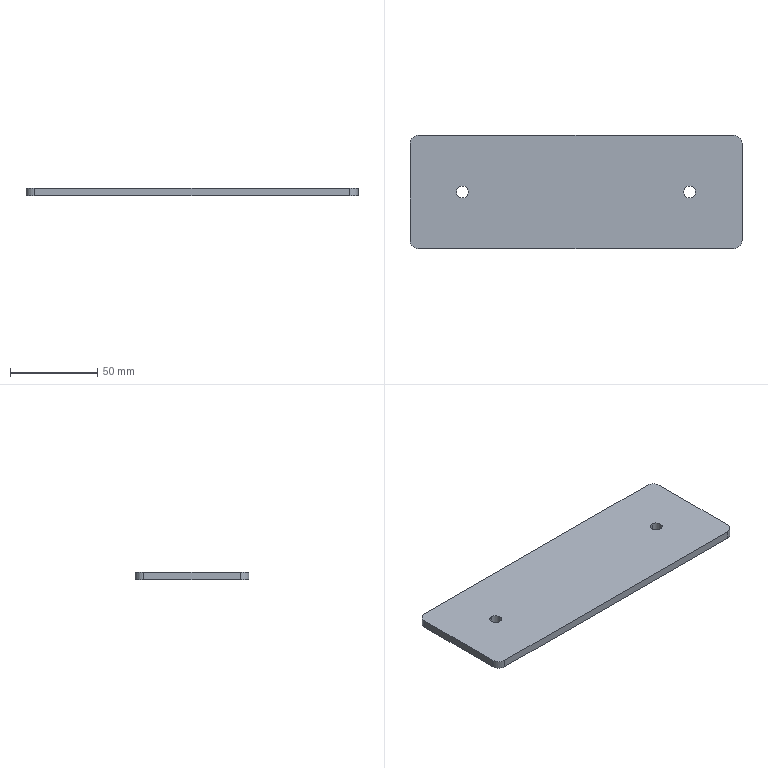Part | STEP file | J452-EBZ05-17-00-Part-1 | 1 solid | 14 faces | box 190 x 65 x 4.5 mm | volume 55152 mm3 | cylinder 8 | plane 6 | commonest cylinder face diameters 6.8 x4 10 x4
STEP:
#1=CARTESIAN_POINT('',(0.,0.,0.));
#2=DIRECTION('',(0.,0.,1.));
#3=DIRECTION('',(1.,0.,0.));
#4=AXIS2_PLACEMENT_3D('',#1,#2,#3);
#5=CARTESIAN_POINT('',(160.,35.9,4.5));
#6=VERTEX_POINT('',#5);
#7=CARTESIAN_POINT('',(160.,35.9,0.));
#8=VERTEX_POINT('',#7);
#9=CARTESIAN_POINT('',(160.,35.9,4.5));
#10=DIRECTION('',(0.,0.,-1.));
#11=VECTOR('',#10,1.);
#12=LINE('',#9,#11);
#13=CARTESIAN_POINT('',(160.,32.5,4.5));
#14=DIRECTION('',(0.,0.,-1.));
#15=DIRECTION('',(0.,1.,0.));
#16=AXIS2_PLACEMENT_3D('',#13,#14,#15);
#17=CYLINDRICAL_SURFACE('',#16,3.4);
#18=CARTESIAN_POINT('',(6.283,0.));
#19=DIRECTION('',(0.,1.));
#20=VECTOR('',#19,1.);
#21=LINE('',#18,#20);
#22=(GEOMETRIC_REPRESENTATION_CONTEXT(2)PARAMETRIC_REPRESENTATION_CONTEXT()REPRESENTATION_CONTEXT('',''));
#23=DEFINITIONAL_REPRESENTATION('',(#21),#22);
#24=PCURVE('',#17,#23);
#25=CARTESIAN_POINT('',(160.,32.5,4.5));
#26=DIRECTION('',(0.,0.,-1.));
#27=DIRECTION('',(0.,1.,0.));
#28=AXIS2_PLACEMENT_3D('',#25,#26,#27);
#29=CYLINDRICAL_SURFACE('',#28,3.4);
#30=CARTESIAN_POINT('',(0.,0.));
#31=DIRECTION('',(0.,1.));
#32=VECTOR('',#31,1.);
#33=LINE('',#30,#32);
#34=(GEOMETRIC_REPRESENTATION_CONTEXT(2)PARAMETRIC_REPRESENTATION_CONTEXT()REPRESENTATION_CONTEXT('',''));
#35=DEFINITIONAL_REPRESENTATION('',(#33),#34);
#36=PCURVE('',#29,#35);
#37=SURFACE_CURVE('',#12,(#24,#36),.PCURVE_S1.);
#38=EDGE_CURVE('',#6,#8,#37,.T.);
#39=ORIENTED_EDGE('',*,*,#38,.T.);
#40=CARTESIAN_POINT('',(160.,29.1,0.));
#41=VERTEX_POINT('',#40);
#42=CARTESIAN_POINT('',(160.,32.5,0.));
#43=DIRECTION('',(0.,0.,1.));
#44=DIRECTION('',(0.,-1.,0.));
#45=AXIS2_PLACEMENT_3D('',#42,#43,#44);
#46=CIRCLE('',#45,3.4);
#47=CARTESIAN_POINT('',(9.425,4.5));
#48=DIRECTION('',(-1.,0.));
#49=VECTOR('',#48,1.);
#50=LINE('',#47,#49);
#51=(GEOMETRIC_REPRESENTATION_CONTEXT(2)PARAMETRIC_REPRESENTATION_CONTEXT()REPRESENTATION_CONTEXT('',''));
#52=DEFINITIONAL_REPRESENTATION('',(#50),#51);
#53=PCURVE('',#17,#52);
#54=CARTESIAN_POINT('',(95.,32.5,0.));
#55=DIRECTION('',(0.,0.,-1.));
#56=DIRECTION('',(0.,1.,0.));
#57=AXIS2_PLACEMENT_3D('',#54,#55,#56);
#58=PLANE('',#57);
#59=CARTESIAN_POINT('',(-3.4,65.));
#60=CARTESIAN_POINT('',(-3.4,70.889));
#61=CARTESIAN_POINT('',(1.7,67.944));
#62=CARTESIAN_POINT('',(6.8,65.));
#63=CARTESIAN_POINT('',(1.7,62.056));
#64=CARTESIAN_POINT('',(-3.4,59.111));
#65=CARTESIAN_POINT('',(-3.4,65.));
#66=(BOUNDED_CURVE()B_SPLINE_CURVE(2,(#59,#60,#61,#62,#63,#64,#65),.UNSPECIFIED.,.T.,.F.)B_SPLINE_CURVE_WITH_KNOTS((1,2,2,2,2,1),(-2.094,0.,2.094,4.189,6.283,8.378),.UNSPECIFIED.)CURVE()GEOMETRIC_REPRESENTATION_ITEM()RATIONAL_B_SPLINE_CURVE((1.,0.5,1.,0.5,1.,0.5,1.))REPRESENTATION_ITEM(''));
#67=(GEOMETRIC_REPRESENTATION_CONTEXT(2)PARAMETRIC_REPRESENTATION_CONTEXT()REPRESENTATION_CONTEXT('',''));
#68=DEFINITIONAL_REPRESENTATION('',(#66),#67);
#69=PCURVE('',#58,#68);
#70=SURFACE_CURVE('',#46,(#53,#69),.PCURVE_S1.);
#71=EDGE_CURVE('',#8,#41,#70,.T.);
#72=ORIENTED_EDGE('',*,*,#71,.T.);
#73=CARTESIAN_POINT('',(160.,29.1,4.5));
#74=VERTEX_POINT('',#73);
#75=CARTESIAN_POINT('',(160.,29.1,4.5));
#76=DIRECTION('',(0.,0.,-1.));
#77=VECTOR('',#76,1.);
#78=LINE('',#75,#77);
#79=CARTESIAN_POINT('',(3.142,0.));
#80=DIRECTION('',(0.,1.));
#81=VECTOR('',#80,1.);
#82=LINE('',#79,#81);
#83=(GEOMETRIC_REPRESENTATION_CONTEXT(2)PARAMETRIC_REPRESENTATION_CONTEXT()REPRESENTATION_CONTEXT('',''));
#84=DEFINITIONAL_REPRESENTATION('',(#82),#83);
#85=PCURVE('',#17,#84);
#86=CARTESIAN_POINT('',(3.142,0.));
#87=DIRECTION('',(0.,1.));
#88=VECTOR('',#87,1.);
#89=LINE('',#86,#88);
#90=(GEOMETRIC_REPRESENTATION_CONTEXT(2)PARAMETRIC_REPRESENTATION_CONTEXT()REPRESENTATION_CONTEXT('',''));
#91=DEFINITIONAL_REPRESENTATION('',(#89),#90);
#92=PCURVE('',#29,#91);
#93=SURFACE_CURVE('',#78,(#85,#92),.PCURVE_S1.);
#94=EDGE_CURVE('',#74,#41,#93,.T.);
#95=ORIENTED_EDGE('',*,*,#94,.F.);
#96=CARTESIAN_POINT('',(160.,32.5,4.5));
#97=DIRECTION('',(0.,0.,-1.));
#98=DIRECTION('',(0.,1.,0.));
#99=AXIS2_PLACEMENT_3D('',#96,#97,#98);
#100=CIRCLE('',#99,3.4);
#101=CARTESIAN_POINT('',(0.,0.));
#102=DIRECTION('',(1.,0.));
#103=VECTOR('',#102,1.);
#104=LINE('',#101,#103);
#105=(GEOMETRIC_REPRESENTATION_CONTEXT(2)PARAMETRIC_REPRESENTATION_CONTEXT()REPRESENTATION_CONTEXT('',''));
#106=DEFINITIONAL_REPRESENTATION('',(#104),#105);
#107=PCURVE('',#17,#106);
#108=CARTESIAN_POINT('',(95.,32.5,4.5));
#109=DIRECTION('',(0.,0.,1.));
#110=DIRECTION('',(0.,-1.,0.));
#111=AXIS2_PLACEMENT_3D('',#108,#109,#110);
#112=PLANE('',#111);
#113=CARTESIAN_POINT('',(-3.4,65.));
#114=CARTESIAN_POINT('',(-3.4,70.889));
#115=CARTESIAN_POINT('',(1.7,67.944));
#116=CARTESIAN_POINT('',(6.8,65.));
#117=CARTESIAN_POINT('',(1.7,62.056));
#118=CARTESIAN_POINT('',(-3.4,59.111));
#119=CARTESIAN_POINT('',(-3.4,65.));
#120=(BOUNDED_CURVE()B_SPLINE_CURVE(2,(#113,#114,#115,#116,#117,#118,#119),.UNSPECIFIED.,.T.,.F.)B_SPLINE_CURVE_WITH_KNOTS((1,2,2,2,2,1),(-2.094,0.,2.094,4.189,6.283,8.378),.UNSPECIFIED.)CURVE()GEOMETRIC_REPRESENTATION_ITEM()RATIONAL_B_SPLINE_CURVE((1.,0.5,1.,0.5,1.,0.5,1.))REPRESENTATION_ITEM(''));
#121=(GEOMETRIC_REPRESENTATION_CONTEXT(2)PARAMETRIC_REPRESENTATION_CONTEXT()REPRESENTATION_CONTEXT('',''));
#122=DEFINITIONAL_REPRESENTATION('',(#120),#121);
#123=PCURVE('',#112,#122);
#124=SURFACE_CURVE('',#100,(#107,#123),.PCURVE_S1.);
#125=EDGE_CURVE('',#74,#6,#124,.T.);
#126=ORIENTED_EDGE('',*,*,#125,.T.);
#127=EDGE_LOOP('',(#39,#72,#95,#126));
#128=FACE_BOUND('',#127,.F.);
#129=ADVANCED_FACE('',(#128),#17,.F.);
#130=CARTESIAN_POINT('',(30.,35.9,4.5));
#131=VERTEX_POINT('',#130);
#132=CARTESIAN_POINT('',(30.,35.9,0.));
#133=VERTEX_POINT('',#132);
#134=CARTESIAN_POINT('',(30.,35.9,4.5));
#135=DIRECTION('',(0.,0.,-1.));
#136=VECTOR('',#135,1.);
#137=LINE('',#134,#136);
#138=CARTESIAN_POINT('',(30.,32.5,4.5));
#139=DIRECTION('',(0.,0.,-1.));
#140=DIRECTION('',(0.,1.,0.));
#141=AXIS2_PLACEMENT_3D('',#138,#139,#140);
#142=CYLINDRICAL_SURFACE('',#141,3.4);
#143=CARTESIAN_POINT('',(6.283,0.));
#144=DIRECTION('',(0.,1.));
#145=VECTOR('',#144,1.);
#146=LINE('',#143,#145);
#147=(GEOMETRIC_REPRESENTATION_CONTEXT(2)PARAMETRIC_REPRESENTATION_CONTEXT()REPRESENTATION_CONTEXT('',''));
#148=DEFINITIONAL_REPRESENTATION('',(#146),#147);
#149=PCURVE('',#142,#148);
#150=CARTESIAN_POINT('',(30.,32.5,4.5));
#151=DIRECTION('',(0.,0.,-1.));
#152=DIRECTION('',(0.,1.,0.));
#153=AXIS2_PLACEMENT_3D('',#150,#151,#152);
#154=CYLINDRICAL_SURFACE('',#153,3.4);
#155=CARTESIAN_POINT('',(0.,0.));
#156=DIRECTION('',(0.,1.));
#157=VECTOR('',#156,1.);
#158=LINE('',#155,#157);
#159=(GEOMETRIC_REPRESENTATION_CONTEXT(2)PARAMETRIC_REPRESENTATION_CONTEXT()REPRESENTATION_CONTEXT('',''));
#160=DEFINITIONAL_REPRESENTATION('',(#158),#159);
#161=PCURVE('',#154,#160);
#162=SURFACE_CURVE('',#137,(#149,#161),.PCURVE_S1.);
#163=EDGE_CURVE('',#131,#133,#162,.T.);
#164=ORIENTED_EDGE('',*,*,#163,.T.);
#165=CARTESIAN_POINT('',(30.,29.1,0.));
#166=VERTEX_POINT('',#165);
#167=CARTESIAN_POINT('',(30.,32.5,0.));
#168=DIRECTION('',(0.,0.,1.));
#169=DIRECTION('',(0.,-1.,0.));
#170=AXIS2_PLACEMENT_3D('',#167,#168,#169);
#171=CIRCLE('',#170,3.4);
#172=CARTESIAN_POINT('',(9.425,4.5));
#173=DIRECTION('',(-1.,0.));
#174=VECTOR('',#173,1.);
#175=LINE('',#172,#174);
#176=(GEOMETRIC_REPRESENTATION_CONTEXT(2)PARAMETRIC_REPRESENTATION_CONTEXT()REPRESENTATION_CONTEXT('',''));
#177=DEFINITIONAL_REPRESENTATION('',(#175),#176);
#178=PCURVE('',#142,#177);
#179=CARTESIAN_POINT('',(-3.4,-65.));
#180=CARTESIAN_POINT('',(-3.4,-59.111));
#181=CARTESIAN_POINT('',(1.7,-62.056));
#182=CARTESIAN_POINT('',(6.8,-65.));
#183=CARTESIAN_POINT('',(1.7,-67.944));
#184=CARTESIAN_POINT('',(-3.4,-70.889));
#185=CARTESIAN_POINT('',(-3.4,-65.));
#186=(BOUNDED_CURVE()B_SPLINE_CURVE(2,(#179,#180,#181,#182,#183,#184,#185),.UNSPECIFIED.,.T.,.F.)B_SPLINE_CURVE_WITH_KNOTS((1,2,2,2,2,1),(-2.094,0.,2.094,4.189,6.283,8.378),.UNSPECIFIED.)CURVE()GEOMETRIC_REPRESENTATION_ITEM()RATIONAL_B_SPLINE_CURVE((1.,0.5,1.,0.5,1.,0.5,1.))REPRESENTATION_ITEM(''));
#187=(GEOMETRIC_REPRESENTATION_CONTEXT(2)PARAMETRIC_REPRESENTATION_CONTEXT()REPRESENTATION_CONTEXT('',''));
#188=DEFINITIONAL_REPRESENTATION('',(#186),#187);
#189=PCURVE('',#58,#188);
#190=SURFACE_CURVE('',#171,(#178,#189),.PCURVE_S1.);
#191=EDGE_CURVE('',#133,#166,#190,.T.);
#192=ORIENTED_EDGE('',*,*,#191,.T.);
#193=CARTESIAN_POINT('',(30.,29.1,4.5));
#194=VERTEX_POINT('',#193);
#195=CARTESIAN_POINT('',(30.,29.1,4.5));
#196=DIRECTION('',(0.,0.,-1.));
#197=VECTOR('',#196,1.);
#198=LINE('',#195,#197);
#199=CARTESIAN_POINT('',(3.142,0.));
#200=DIRECTION('',(0.,1.));
#201=VECTOR('',#200,1.);
#202=LINE('',#199,#201);
#203=(GEOMETRIC_REPRESENTATION_CONTEXT(2)PARAMETRIC_REPRESENTATION_CONTEXT()REPRESENTATION_CONTEXT('',''));
#204=DEFINITIONAL_REPRESENTATION('',(#202),#203);
#205=PCURVE('',#142,#204);
#206=CARTESIAN_POINT('',(3.142,0.));
#207=DIRECTION('',(0.,1.));
#208=VECTOR('',#207,1.);
#209=LINE('',#206,#208);
#210=(GEOMETRIC_REPRESENTATION_CONTEXT(2)PARAMETRIC_REPRESENTATION_CONTEXT()REPRESENTATION_CONTEXT('',''));
#211=DEFINITIONAL_REPRESENTATION('',(#209),#210);
#212=PCURVE('',#154,#211);
#213=SURFACE_CURVE('',#198,(#205,#212),.PCURVE_S1.);
#214=EDGE_CURVE('',#194,#166,#213,.T.);
#215=ORIENTED_EDGE('',*,*,#214,.F.);
#216=CARTESIAN_POINT('',(30.,32.5,4.5));
#217=DIRECTION('',(0.,0.,-1.));
#218=DIRECTION('',(0.,1.,0.));
#219=AXIS2_PLACEMENT_3D('',#216,#217,#218);
#220=CIRCLE('',#219,3.4);
#221=CARTESIAN_POINT('',(0.,0.));
#222=DIRECTION('',(1.,0.));
#223=VECTOR('',#222,1.);
#224=LINE('',#221,#223);
#225=(GEOMETRIC_REPRESENTATION_CONTEXT(2)PARAMETRIC_REPRESENTATION_CONTEXT()REPRESENTATION_CONTEXT('',''));
#226=DEFINITIONAL_REPRESENTATION('',(#224),#225);
#227=PCURVE('',#142,#226);
#228=CARTESIAN_POINT('',(-3.4,-65.));
#229=CARTESIAN_POINT('',(-3.4,-59.111));
#230=CARTESIAN_POINT('',(1.7,-62.056));
#231=CARTESIAN_POINT('',(6.8,-65.));
#232=CARTESIAN_POINT('',(1.7,-67.944));
#233=CARTESIAN_POINT('',(-3.4,-70.889));
#234=CARTESIAN_POINT('',(-3.4,-65.));
#235=(BOUNDED_CURVE()B_SPLINE_CURVE(2,(#228,#229,#230,#231,#232,#233,#234),.UNSPECIFIED.,.T.,.F.)B_SPLINE_CURVE_WITH_KNOTS((1,2,2,2,2,1),(-2.094,0.,2.094,4.189,6.283,8.378),.UNSPECIFIED.)CURVE()GEOMETRIC_REPRESENTATION_ITEM()RATIONAL_B_SPLINE_CURVE((1.,0.5,1.,0.5,1.,0.5,1.))REPRESENTATION_ITEM(''));
#236=(GEOMETRIC_REPRESENTATION_CONTEXT(2)PARAMETRIC_REPRESENTATION_CONTEXT()REPRESENTATION_CONTEXT('',''));
#237=DEFINITIONAL_REPRESENTATION('',(#235),#236);
#238=PCURVE('',#112,#237);
#239=SURFACE_CURVE('',#220,(#227,#238),.PCURVE_S1.);
#240=EDGE_CURVE('',#194,#131,#239,.T.);
#241=ORIENTED_EDGE('',*,*,#240,.T.);
#242=EDGE_LOOP('',(#164,#192,#215,#241));
#243=FACE_BOUND('',#242,.F.);
#244=ADVANCED_FACE('',(#243),#142,.F.);
#245=CARTESIAN_POINT('',(160.,32.5,4.5));
#246=DIRECTION('',(0.,0.,-1.));
#247=DIRECTION('',(0.,1.,0.));
#248=AXIS2_PLACEMENT_3D('',#245,#246,#247);
#249=CIRCLE('',#248,3.4);
#250=CARTESIAN_POINT('',(-3.4,65.));
#251=CARTESIAN_POINT('',(-3.4,70.889));
#252=CARTESIAN_POINT('',(1.7,67.944));
#253=CARTESIAN_POINT('',(6.8,65.));
#254=CARTESIAN_POINT('',(1.7,62.056));
#255=CARTESIAN_POINT('',(-3.4,59.111));
#256=CARTESIAN_POINT('',(-3.4,65.));
#257=(BOUNDED_CURVE()B_SPLINE_CURVE(2,(#250,#251,#252,#253,#254,#255,#256),.UNSPECIFIED.,.T.,.F.)B_SPLINE_CURVE_WITH_KNOTS((1,2,2,2,2,1),(-2.094,0.,2.094,4.189,6.283,8.378),.UNSPECIFIED.)CURVE()GEOMETRIC_REPRESENTATION_ITEM()RATIONAL_B_SPLINE_CURVE((1.,0.5,1.,0.5,1.,0.5,1.))REPRESENTATION_ITEM(''));
#258=(GEOMETRIC_REPRESENTATION_CONTEXT(2)PARAMETRIC_REPRESENTATION_CONTEXT()REPRESENTATION_CONTEXT('',''));
#259=DEFINITIONAL_REPRESENTATION('',(#257),#258);
#260=PCURVE('',#112,#259);
#261=CARTESIAN_POINT('',(0.,0.));
#262=DIRECTION('',(1.,0.));
#263=VECTOR('',#262,1.);
#264=LINE('',#261,#263);
#265=(GEOMETRIC_REPRESENTATION_CONTEXT(2)PARAMETRIC_REPRESENTATION_CONTEXT()REPRESENTATION_CONTEXT('',''));
#266=DEFINITIONAL_REPRESENTATION('',(#264),#265);
#267=PCURVE('',#29,#266);
#268=SURFACE_CURVE('',#249,(#260,#267),.PCURVE_S1.);
#269=EDGE_CURVE('',#6,#74,#268,.T.);
#270=ORIENTED_EDGE('',*,*,#269,.T.);
#271=ORIENTED_EDGE('',*,*,#125,.T.);
#272=EDGE_LOOP('',(#270,#271));
#273=FACE_BOUND('',#272,.T.);
#274=CARTESIAN_POINT('',(30.,32.5,4.5));
#275=DIRECTION('',(0.,0.,-1.));
#276=DIRECTION('',(0.,1.,0.));
#277=AXIS2_PLACEMENT_3D('',#274,#275,#276);
#278=CIRCLE('',#277,3.4);
#279=CARTESIAN_POINT('',(-3.4,-65.));
#280=CARTESIAN_POINT('',(-3.4,-59.111));
#281=CARTESIAN_POINT('',(1.7,-62.056));
#282=CARTESIAN_POINT('',(6.8,-65.));
#283=CARTESIAN_POINT('',(1.7,-67.944));
#284=CARTESIAN_POINT('',(-3.4,-70.889));
#285=CARTESIAN_POINT('',(-3.4,-65.));
#286=(BOUNDED_CURVE()B_SPLINE_CURVE(2,(#279,#280,#281,#282,#283,#284,#285),.UNSPECIFIED.,.T.,.F.)B_SPLINE_CURVE_WITH_KNOTS((1,2,2,2,2,1),(-2.094,0.,2.094,4.189,6.283,8.378),.UNSPECIFIED.)CURVE()GEOMETRIC_REPRESENTATION_ITEM()RATIONAL_B_SPLINE_CURVE((1.,0.5,1.,0.5,1.,0.5,1.))REPRESENTATION_ITEM(''));
#287=(GEOMETRIC_REPRESENTATION_CONTEXT(2)PARAMETRIC_REPRESENTATION_CONTEXT()REPRESENTATION_CONTEXT('',''));
#288=DEFINITIONAL_REPRESENTATION('',(#286),#287);
#289=PCURVE('',#112,#288);
#290=CARTESIAN_POINT('',(0.,0.));
#291=DIRECTION('',(1.,0.));
#292=VECTOR('',#291,1.);
#293=LINE('',#290,#292);
#294=(GEOMETRIC_REPRESENTATION_CONTEXT(2)PARAMETRIC_REPRESENTATION_CONTEXT()REPRESENTATION_CONTEXT('',''));
#295=DEFINITIONAL_REPRESENTATION('',(#293),#294);
#296=PCURVE('',#154,#295);
#297=SURFACE_CURVE('',#278,(#289,#296),.PCURVE_S1.);
#298=EDGE_CURVE('',#131,#194,#297,.T.);
#299=ORIENTED_EDGE('',*,*,#298,.T.);
#300=ORIENTED_EDGE('',*,*,#240,.T.);
#301=EDGE_LOOP('',(#299,#300));
#302=FACE_BOUND('',#301,.T.);
#303=CARTESIAN_POINT('',(5.,65.,4.5));
#304=VERTEX_POINT('',#303);
#305=CARTESIAN_POINT('',(185.,65.,4.5));
#306=VERTEX_POINT('',#305);
#307=CARTESIAN_POINT('',(95.,65.,4.5));
#308=DIRECTION('',(1.,0.,0.));
#309=VECTOR('',#308,1.);
#310=LINE('',#307,#309);
#311=CARTESIAN_POINT('',(-32.5,0.));
#312=DIRECTION('',(0.,1.));
#313=VECTOR('',#312,1.);
#314=LINE('',#311,#313);
#315=(GEOMETRIC_REPRESENTATION_CONTEXT(2)PARAMETRIC_REPRESENTATION_CONTEXT()REPRESENTATION_CONTEXT('',''));
#316=DEFINITIONAL_REPRESENTATION('',(#314),#315);
#317=PCURVE('',#112,#316);
#318=CARTESIAN_POINT('',(95.,65.,0.));
#319=DIRECTION('',(0.,1.,0.));
#320=DIRECTION('',(0.,0.,1.));
#321=AXIS2_PLACEMENT_3D('',#318,#319,#320);
#322=PLANE('',#321);
#323=CARTESIAN_POINT('',(4.5,0.));
#324=DIRECTION('',(0.,1.));
#325=VECTOR('',#324,1.);
#326=LINE('',#323,#325);
#327=(GEOMETRIC_REPRESENTATION_CONTEXT(2)PARAMETRIC_REPRESENTATION_CONTEXT()REPRESENTATION_CONTEXT('',''));
#328=DEFINITIONAL_REPRESENTATION('',(#326),#327);
#329=PCURVE('',#322,#328);
#330=SURFACE_CURVE('',#310,(#317,#329),.PCURVE_S1.);
#331=EDGE_CURVE('',#304,#306,#330,.T.);
#332=ORIENTED_EDGE('',*,*,#331,.F.);
#333=CARTESIAN_POINT('',(0.,60.,4.5));
#334=VERTEX_POINT('',#333);
#335=CARTESIAN_POINT('',(5.,60.,4.5));
#336=DIRECTION('',(0.,0.,1.));
#337=DIRECTION('',(0.,-1.,0.));
#338=AXIS2_PLACEMENT_3D('',#335,#336,#337);
#339=CIRCLE('',#338,5.);
#340=CARTESIAN_POINT('',(-27.5,-90.));
#341=DIRECTION('',(1.,0.));
#342=AXIS2_PLACEMENT_2D('',#340,#341);
#343=CIRCLE('',#342,5.);
#344=(GEOMETRIC_REPRESENTATION_CONTEXT(2)PARAMETRIC_REPRESENTATION_CONTEXT()REPRESENTATION_CONTEXT('',''));
#345=DEFINITIONAL_REPRESENTATION('',(#343),#344);
#346=PCURVE('',#112,#345);
#347=CARTESIAN_POINT('',(5.,60.,0.));
#348=DIRECTION('',(0.,0.,1.));
#349=DIRECTION('',(0.,-1.,0.));
#350=AXIS2_PLACEMENT_3D('',#347,#348,#349);
#351=CYLINDRICAL_SURFACE('',#350,5.);
#352=CARTESIAN_POINT('',(0.,4.5));
#353=DIRECTION('',(1.,0.));
#354=VECTOR('',#353,1.);
#355=LINE('',#352,#354);
#356=(GEOMETRIC_REPRESENTATION_CONTEXT(2)PARAMETRIC_REPRESENTATION_CONTEXT()REPRESENTATION_CONTEXT('',''));
#357=DEFINITIONAL_REPRESENTATION('',(#355),#356);
#358=PCURVE('',#351,#357);
#359=SURFACE_CURVE('',#339,(#346,#358),.PCURVE_S1.);
#360=EDGE_CURVE('',#304,#334,#359,.T.);
#361=ORIENTED_EDGE('',*,*,#360,.T.);
#362=CARTESIAN_POINT('',(0.,5.,4.5));
#363=VERTEX_POINT('',#362);
#364=CARTESIAN_POINT('',(0.,32.5,4.5));
#365=DIRECTION('',(0.,1.,0.));
#366=VECTOR('',#365,1.);
#367=LINE('',#364,#366);
#368=CARTESIAN_POINT('',(0.,-95.));
#369=DIRECTION('',(-1.,0.));
#370=VECTOR('',#369,1.);
#371=LINE('',#368,#370);
#372=(GEOMETRIC_REPRESENTATION_CONTEXT(2)PARAMETRIC_REPRESENTATION_CONTEXT()REPRESENTATION_CONTEXT('',''));
#373=DEFINITIONAL_REPRESENTATION('',(#371),#372);
#374=PCURVE('',#112,#373);
#375=CARTESIAN_POINT('',(0.,32.5,0.));
#376=DIRECTION('',(-1.,0.,0.));
#377=DIRECTION('',(0.,0.,-1.));
#378=AXIS2_PLACEMENT_3D('',#375,#376,#377);
#379=PLANE('',#378);
#380=CARTESIAN_POINT('',(-4.5,0.));
#381=DIRECTION('',(0.,-1.));
#382=VECTOR('',#381,1.);
#383=LINE('',#380,#382);
#384=(GEOMETRIC_REPRESENTATION_CONTEXT(2)PARAMETRIC_REPRESENTATION_CONTEXT()REPRESENTATION_CONTEXT('',''));
#385=DEFINITIONAL_REPRESENTATION('',(#383),#384);
#386=PCURVE('',#379,#385);
#387=SURFACE_CURVE('',#367,(#374,#386),.PCURVE_S1.);
#388=EDGE_CURVE('',#363,#334,#387,.T.);
#389=ORIENTED_EDGE('',*,*,#388,.F.);
#390=CARTESIAN_POINT('',(5.,0.,4.5));
#391=VERTEX_POINT('',#390);
#392=CARTESIAN_POINT('',(5.,5.,4.5));
#393=DIRECTION('',(0.,0.,1.));
#394=DIRECTION('',(0.,-1.,0.));
#395=AXIS2_PLACEMENT_3D('',#392,#393,#394);
#396=CIRCLE('',#395,5.);
#397=CARTESIAN_POINT('',(27.5,-90.));
#398=DIRECTION('',(1.,0.));
#399=AXIS2_PLACEMENT_2D('',#397,#398);
#400=CIRCLE('',#399,5.);
#401=(GEOMETRIC_REPRESENTATION_CONTEXT(2)PARAMETRIC_REPRESENTATION_CONTEXT()REPRESENTATION_CONTEXT('',''));
#402=DEFINITIONAL_REPRESENTATION('',(#400),#401);
#403=PCURVE('',#112,#402);
#404=CARTESIAN_POINT('',(5.,5.,0.));
#405=DIRECTION('',(0.,0.,1.));
#406=DIRECTION('',(0.,-1.,0.));
#407=AXIS2_PLACEMENT_3D('',#404,#405,#406);
#408=CYLINDRICAL_SURFACE('',#407,5.);
#409=CARTESIAN_POINT('',(0.,4.5));
#410=DIRECTION('',(1.,0.));
#411=VECTOR('',#410,1.);
#412=LINE('',#409,#411);
#413=(GEOMETRIC_REPRESENTATION_CONTEXT(2)PARAMETRIC_REPRESENTATION_CONTEXT()REPRESENTATION_CONTEXT('',''));
#414=DEFINITIONAL_REPRESENTATION('',(#412),#413);
#415=PCURVE('',#408,#414);
#416=SURFACE_CURVE('',#396,(#403,#415),.PCURVE_S1.);
#417=EDGE_CURVE('',#363,#391,#416,.T.);
#418=ORIENTED_EDGE('',*,*,#417,.T.);
#419=CARTESIAN_POINT('',(185.,0.,4.5));
#420=VERTEX_POINT('',#419);
#421=CARTESIAN_POINT('',(95.,0.,4.5));
#422=DIRECTION('',(-1.,0.,0.));
#423=VECTOR('',#422,1.);
#424=LINE('',#421,#423);
#425=CARTESIAN_POINT('',(32.5,0.));
#426=DIRECTION('',(0.,-1.));
#427=VECTOR('',#426,1.);
#428=LINE('',#425,#427);
#429=(GEOMETRIC_REPRESENTATION_CONTEXT(2)PARAMETRIC_REPRESENTATION_CONTEXT()REPRESENTATION_CONTEXT('',''));
#430=DEFINITIONAL_REPRESENTATION('',(#428),#429);
#431=PCURVE('',#112,#430);
#432=CARTESIAN_POINT('',(95.,0.,0.));
#433=DIRECTION('',(0.,-1.,0.));
#434=DIRECTION('',(0.,0.,-1.));
#435=AXIS2_PLACEMENT_3D('',#432,#433,#434);
#436=PLANE('',#435);
#437=CARTESIAN_POINT('',(-4.5,0.));
#438=DIRECTION('',(0.,-1.));
#439=VECTOR('',#438,1.);
#440=LINE('',#437,#439);
#441=(GEOMETRIC_REPRESENTATION_CONTEXT(2)PARAMETRIC_REPRESENTATION_CONTEXT()REPRESENTATION_CONTEXT('',''));
#442=DEFINITIONAL_REPRESENTATION('',(#440),#441);
#443=PCURVE('',#436,#442);
#444=SURFACE_CURVE('',#424,(#431,#443),.PCURVE_S1.);
#445=EDGE_CURVE('',#420,#391,#444,.T.);
#446=ORIENTED_EDGE('',*,*,#445,.F.);
#447=CARTESIAN_POINT('',(190.,5.,4.5));
#448=VERTEX_POINT('',#447);
#449=CARTESIAN_POINT('',(185.,5.,4.5));
#450=DIRECTION('',(0.,0.,1.));
#451=DIRECTION('',(0.,-1.,0.));
#452=AXIS2_PLACEMENT_3D('',#449,#450,#451);
#453=CIRCLE('',#452,5.);
#454=CARTESIAN_POINT('',(27.5,90.));
#455=DIRECTION('',(1.,0.));
#456=AXIS2_PLACEMENT_2D('',#454,#455);
#457=CIRCLE('',#456,5.);
#458=(GEOMETRIC_REPRESENTATION_CONTEXT(2)PARAMETRIC_REPRESENTATION_CONTEXT()REPRESENTATION_CONTEXT('',''));
#459=DEFINITIONAL_REPRESENTATION('',(#457),#458);
#460=PCURVE('',#112,#459);
#461=CARTESIAN_POINT('',(185.,5.,0.));
#462=DIRECTION('',(0.,0.,1.));
#463=DIRECTION('',(0.,-1.,0.));
#464=AXIS2_PLACEMENT_3D('',#461,#462,#463);
#465=CYLINDRICAL_SURFACE('',#464,5.);
#466=CARTESIAN_POINT('',(0.,4.5));
#467=DIRECTION('',(1.,0.));
#468=VECTOR('',#467,1.);
#469=LINE('',#466,#468);
#470=(GEOMETRIC_REPRESENTATION_CONTEXT(2)PARAMETRIC_REPRESENTATION_CONTEXT()REPRESENTATION_CONTEXT('',''));
#471=DEFINITIONAL_REPRESENTATION('',(#469),#470);
#472=PCURVE('',#465,#471);
#473=SURFACE_CURVE('',#453,(#460,#472),.PCURVE_S1.);
#474=EDGE_CURVE('',#420,#448,#473,.T.);
#475=ORIENTED_EDGE('',*,*,#474,.T.);
#476=CARTESIAN_POINT('',(190.,60.,4.5));
#477=VERTEX_POINT('',#476);
#478=CARTESIAN_POINT('',(190.,32.5,4.5));
#479=DIRECTION('',(0.,-1.,0.));
#480=VECTOR('',#479,1.);
#481=LINE('',#478,#480);
#482=CARTESIAN_POINT('',(0.,95.));
#483=DIRECTION('',(1.,0.));
#484=VECTOR('',#483,1.);
#485=LINE('',#482,#484);
#486=(GEOMETRIC_REPRESENTATION_CONTEXT(2)PARAMETRIC_REPRESENTATION_CONTEXT()REPRESENTATION_CONTEXT('',''));
#487=DEFINITIONAL_REPRESENTATION('',(#485),#486);
#488=PCURVE('',#112,#487);
#489=CARTESIAN_POINT('',(190.,32.5,0.));
#490=DIRECTION('',(1.,0.,0.));
#491=DIRECTION('',(0.,0.,1.));
#492=AXIS2_PLACEMENT_3D('',#489,#490,#491);
#493=PLANE('',#492);
#494=CARTESIAN_POINT('',(4.5,0.));
#495=DIRECTION('',(0.,1.));
#496=VECTOR('',#495,1.);
#497=LINE('',#494,#496);
#498=(GEOMETRIC_REPRESENTATION_CONTEXT(2)PARAMETRIC_REPRESENTATION_CONTEXT()REPRESENTATION_CONTEXT('',''));
#499=DEFINITIONAL_REPRESENTATION('',(#497),#498);
#500=PCURVE('',#493,#499);
#501=SURFACE_CURVE('',#481,(#488,#500),.PCURVE_S1.);
#502=EDGE_CURVE('',#477,#448,#501,.T.);
#503=ORIENTED_EDGE('',*,*,#502,.F.);
#504=CARTESIAN_POINT('',(185.,60.,4.5));
#505=DIRECTION('',(0.,0.,1.));
#506=DIRECTION('',(0.,-1.,0.));
#507=AXIS2_PLACEMENT_3D('',#504,#505,#506);
#508=CIRCLE('',#507,5.);
#509=CARTESIAN_POINT('',(-27.5,90.));
#510=DIRECTION('',(1.,0.));
#511=AXIS2_PLACEMENT_2D('',#509,#510);
#512=CIRCLE('',#511,5.);
#513=(GEOMETRIC_REPRESENTATION_CONTEXT(2)PARAMETRIC_REPRESENTATION_CONTEXT()REPRESENTATION_CONTEXT('',''));
#514=DEFINITIONAL_REPRESENTATION('',(#512),#513);
#515=PCURVE('',#112,#514);
#516=CARTESIAN_POINT('',(185.,60.,0.));
#517=DIRECTION('',(0.,0.,1.));
#518=DIRECTION('',(0.,-1.,0.));
#519=AXIS2_PLACEMENT_3D('',#516,#517,#518);
#520=CYLINDRICAL_SURFACE('',#519,5.);
#521=CARTESIAN_POINT('',(0.,4.5));
#522=DIRECTION('',(1.,0.));
#523=VECTOR('',#522,1.);
#524=LINE('',#521,#523);
#525=(GEOMETRIC_REPRESENTATION_CONTEXT(2)PARAMETRIC_REPRESENTATION_CONTEXT()REPRESENTATION_CONTEXT('',''));
#526=DEFINITIONAL_REPRESENTATION('',(#524),#525);
#527=PCURVE('',#520,#526);
#528=SURFACE_CURVE('',#508,(#515,#527),.PCURVE_S1.);
#529=EDGE_CURVE('',#477,#306,#528,.T.);
#530=ORIENTED_EDGE('',*,*,#529,.T.);
#531=EDGE_LOOP('',(#332,#361,#389,#418,#446,#475,#503,#530));
#532=FACE_BOUND('',#531,.T.);
#533=ADVANCED_FACE('',(#273,#302,#532),#112,.T.);
#534=ORIENTED_EDGE('',*,*,#388,.T.);
#535=CARTESIAN_POINT('',(0.,60.,0.));
#536=VERTEX_POINT('',#535);
#537=CARTESIAN_POINT('',(0.,60.,0.));
#538=DIRECTION('',(0.,0.,-1.));
#539=VECTOR('',#538,1.);
#540=LINE('',#537,#539);
#541=CARTESIAN_POINT('',(0.,-27.5));
#542=DIRECTION('',(1.,0.));
#543=VECTOR('',#542,1.);
#544=LINE('',#541,#543);
#545=(GEOMETRIC_REPRESENTATION_CONTEXT(2)PARAMETRIC_REPRESENTATION_CONTEXT()REPRESENTATION_CONTEXT('',''));
#546=DEFINITIONAL_REPRESENTATION('',(#544),#545);
#547=PCURVE('',#379,#546);
#548=CARTESIAN_POINT('',(4.712,0.));
#549=DIRECTION('',(0.,-1.));
#550=VECTOR('',#549,1.);
#551=LINE('',#548,#550);
#552=(GEOMETRIC_REPRESENTATION_CONTEXT(2)PARAMETRIC_REPRESENTATION_CONTEXT()REPRESENTATION_CONTEXT('',''));
#553=DEFINITIONAL_REPRESENTATION('',(#551),#552);
#554=PCURVE('',#351,#553);
#555=SURFACE_CURVE('',#540,(#547,#554),.PCURVE_S1.);
#556=EDGE_CURVE('',#334,#536,#555,.T.);
#557=ORIENTED_EDGE('',*,*,#556,.T.);
#558=CARTESIAN_POINT('',(0.,5.,0.));
#559=VERTEX_POINT('',#558);
#560=CARTESIAN_POINT('',(0.,32.5,0.));
#561=DIRECTION('',(0.,-1.,0.));
#562=VECTOR('',#561,1.);
#563=LINE('',#560,#562);
#564=CARTESIAN_POINT('',(0.,0.));
#565=DIRECTION('',(0.,1.));
#566=VECTOR('',#565,1.);
#567=LINE('',#564,#566);
#568=(GEOMETRIC_REPRESENTATION_CONTEXT(2)PARAMETRIC_REPRESENTATION_CONTEXT()REPRESENTATION_CONTEXT('',''));
#569=DEFINITIONAL_REPRESENTATION('',(#567),#568);
#570=PCURVE('',#379,#569);
#571=CARTESIAN_POINT('',(0.,-95.));
#572=DIRECTION('',(-1.,0.));
#573=VECTOR('',#572,1.);
#574=LINE('',#571,#573);
#575=(GEOMETRIC_REPRESENTATION_CONTEXT(2)PARAMETRIC_REPRESENTATION_CONTEXT()REPRESENTATION_CONTEXT('',''));
#576=DEFINITIONAL_REPRESENTATION('',(#574),#575);
#577=PCURVE('',#58,#576);
#578=SURFACE_CURVE('',#563,(#570,#577),.PCURVE_S1.);
#579=EDGE_CURVE('',#536,#559,#578,.T.);
#580=ORIENTED_EDGE('',*,*,#579,.T.);
#581=CARTESIAN_POINT('',(0.,5.,0.));
#582=DIRECTION('',(0.,0.,1.));
#583=VECTOR('',#582,1.);
#584=LINE('',#581,#583);
#585=CARTESIAN_POINT('',(0.,27.5));
#586=DIRECTION('',(-1.,0.));
#587=VECTOR('',#586,1.);
#588=LINE('',#585,#587);
#589=(GEOMETRIC_REPRESENTATION_CONTEXT(2)PARAMETRIC_REPRESENTATION_CONTEXT()REPRESENTATION_CONTEXT('',''));
#590=DEFINITIONAL_REPRESENTATION('',(#588),#589);
#591=PCURVE('',#379,#590);
#592=CARTESIAN_POINT('',(4.712,0.));
#593=DIRECTION('',(0.,1.));
#594=VECTOR('',#593,1.);
#595=LINE('',#592,#594);
#596=(GEOMETRIC_REPRESENTATION_CONTEXT(2)PARAMETRIC_REPRESENTATION_CONTEXT()REPRESENTATION_CONTEXT('',''));
#597=DEFINITIONAL_REPRESENTATION('',(#595),#596);
#598=PCURVE('',#408,#597);
#599=SURFACE_CURVE('',#584,(#591,#598),.PCURVE_S1.);
#600=EDGE_CURVE('',#559,#363,#599,.T.);
#601=ORIENTED_EDGE('',*,*,#600,.T.);
#602=EDGE_LOOP('',(#534,#557,#580,#601));
#603=FACE_BOUND('',#602,.T.);
#604=ADVANCED_FACE('',(#603),#379,.T.);
#605=CARTESIAN_POINT('',(185.,65.,0.));
#606=VERTEX_POINT('',#605);
#607=CARTESIAN_POINT('',(5.,65.,0.));
#608=VERTEX_POINT('',#607);
#609=CARTESIAN_POINT('',(95.,65.,0.));
#610=DIRECTION('',(-1.,0.,0.));
#611=VECTOR('',#610,1.);
#612=LINE('',#609,#611);
#613=CARTESIAN_POINT('',(0.,0.));
#614=DIRECTION('',(0.,-1.));
#615=VECTOR('',#614,1.);
#616=LINE('',#613,#615);
#617=(GEOMETRIC_REPRESENTATION_CONTEXT(2)PARAMETRIC_REPRESENTATION_CONTEXT()REPRESENTATION_CONTEXT('',''));
#618=DEFINITIONAL_REPRESENTATION('',(#616),#617);
#619=PCURVE('',#322,#618);
#620=CARTESIAN_POINT('',(32.5,0.));
#621=DIRECTION('',(0.,-1.));
#622=VECTOR('',#621,1.);
#623=LINE('',#620,#622);
#624=(GEOMETRIC_REPRESENTATION_CONTEXT(2)PARAMETRIC_REPRESENTATION_CONTEXT()REPRESENTATION_CONTEXT('',''));
#625=DEFINITIONAL_REPRESENTATION('',(#623),#624);
#626=PCURVE('',#58,#625);
#627=SURFACE_CURVE('',#612,(#619,#626),.PCURVE_S1.);
#628=EDGE_CURVE('',#606,#608,#627,.T.);
#629=ORIENTED_EDGE('',*,*,#628,.T.);
#630=CARTESIAN_POINT('',(5.,65.,0.));
#631=DIRECTION('',(0.,0.,1.));
#632=VECTOR('',#631,1.);
#633=LINE('',#630,#632);
#634=CARTESIAN_POINT('',(0.,-90.));
#635=DIRECTION('',(1.,0.));
#636=VECTOR('',#635,1.);
#637=LINE('',#634,#636);
#638=(GEOMETRIC_REPRESENTATION_CONTEXT(2)PARAMETRIC_REPRESENTATION_CONTEXT()REPRESENTATION_CONTEXT('',''));
#639=DEFINITIONAL_REPRESENTATION('',(#637),#638);
#640=PCURVE('',#322,#639);
#641=CARTESIAN_POINT('',(3.142,0.));
#642=DIRECTION('',(0.,1.));
#643=VECTOR('',#642,1.);
#644=LINE('',#641,#643);
#645=(GEOMETRIC_REPRESENTATION_CONTEXT(2)PARAMETRIC_REPRESENTATION_CONTEXT()REPRESENTATION_CONTEXT('',''));
#646=DEFINITIONAL_REPRESENTATION('',(#644),#645);
#647=PCURVE('',#351,#646);
#648=SURFACE_CURVE('',#633,(#640,#647),.PCURVE_S1.);
#649=EDGE_CURVE('',#608,#304,#648,.T.);
#650=ORIENTED_EDGE('',*,*,#649,.T.);
#651=ORIENTED_EDGE('',*,*,#331,.T.);
#652=CARTESIAN_POINT('',(185.,65.,0.));
#653=DIRECTION('',(0.,0.,-1.));
#654=VECTOR('',#653,1.);
#655=LINE('',#652,#654);
#656=CARTESIAN_POINT('',(0.,90.));
#657=DIRECTION('',(-1.,0.));
#658=VECTOR('',#657,1.);
#659=LINE('',#656,#658);
#660=(GEOMETRIC_REPRESENTATION_CONTEXT(2)PARAMETRIC_REPRESENTATION_CONTEXT()REPRESENTATION_CONTEXT('',''));
#661=DEFINITIONAL_REPRESENTATION('',(#659),#660);
#662=PCURVE('',#322,#661);
#663=CARTESIAN_POINT('',(3.142,0.));
#664=DIRECTION('',(0.,-1.));
#665=VECTOR('',#664,1.);
#666=LINE('',#663,#665);
#667=(GEOMETRIC_REPRESENTATION_CONTEXT(2)PARAMETRIC_REPRESENTATION_CONTEXT()REPRESENTATION_CONTEXT('',''));
#668=DEFINITIONAL_REPRESENTATION('',(#666),#667);
#669=PCURVE('',#520,#668);
#670=SURFACE_CURVE('',#655,(#662,#669),.PCURVE_S1.);
#671=EDGE_CURVE('',#306,#606,#670,.T.);
#672=ORIENTED_EDGE('',*,*,#671,.T.);
#673=EDGE_LOOP('',(#629,#650,#651,#672));
#674=FACE_BOUND('',#673,.T.);
#675=ADVANCED_FACE('',(#674),#322,.T.);
#676=CARTESIAN_POINT('',(190.,5.,0.));
#677=VERTEX_POINT('',#676);
#678=CARTESIAN_POINT('',(190.,60.,0.));
#679=VERTEX_POINT('',#678);
#680=CARTESIAN_POINT('',(190.,32.5,0.));
#681=DIRECTION('',(0.,1.,0.));
#682=VECTOR('',#681,1.);
#683=LINE('',#680,#682);
#684=CARTESIAN_POINT('',(0.,0.));
#685=DIRECTION('',(0.,-1.));
#686=VECTOR('',#685,1.);
#687=LINE('',#684,#686);
#688=(GEOMETRIC_REPRESENTATION_CONTEXT(2)PARAMETRIC_REPRESENTATION_CONTEXT()REPRESENTATION_CONTEXT('',''));
#689=DEFINITIONAL_REPRESENTATION('',(#687),#688);
#690=PCURVE('',#493,#689);
#691=CARTESIAN_POINT('',(0.,95.));
#692=DIRECTION('',(1.,0.));
#693=VECTOR('',#692,1.);
#694=LINE('',#691,#693);
#695=(GEOMETRIC_REPRESENTATION_CONTEXT(2)PARAMETRIC_REPRESENTATION_CONTEXT()REPRESENTATION_CONTEXT('',''));
#696=DEFINITIONAL_REPRESENTATION('',(#694),#695);
#697=PCURVE('',#58,#696);
#698=SURFACE_CURVE('',#683,(#690,#697),.PCURVE_S1.);
#699=EDGE_CURVE('',#677,#679,#698,.T.);
#700=ORIENTED_EDGE('',*,*,#699,.T.);
#701=CARTESIAN_POINT('',(190.,60.,0.));
#702=DIRECTION('',(0.,0.,1.));
#703=VECTOR('',#702,1.);
#704=LINE('',#701,#703);
#705=CARTESIAN_POINT('',(0.,-27.5));
#706=DIRECTION('',(1.,0.));
#707=VECTOR('',#706,1.);
#708=LINE('',#705,#707);
#709=(GEOMETRIC_REPRESENTATION_CONTEXT(2)PARAMETRIC_REPRESENTATION_CONTEXT()REPRESENTATION_CONTEXT('',''));
#710=DEFINITIONAL_REPRESENTATION('',(#708),#709);
#711=PCURVE('',#493,#710);
#712=CARTESIAN_POINT('',(1.571,0.));
#713=DIRECTION('',(0.,1.));
#714=VECTOR('',#713,1.);
#715=LINE('',#712,#714);
#716=(GEOMETRIC_REPRESENTATION_CONTEXT(2)PARAMETRIC_REPRESENTATION_CONTEXT()REPRESENTATION_CONTEXT('',''));
#717=DEFINITIONAL_REPRESENTATION('',(#715),#716);
#718=PCURVE('',#520,#717);
#719=SURFACE_CURVE('',#704,(#711,#718),.PCURVE_S1.);
#720=EDGE_CURVE('',#679,#477,#719,.T.);
#721=ORIENTED_EDGE('',*,*,#720,.T.);
#722=ORIENTED_EDGE('',*,*,#502,.T.);
#723=CARTESIAN_POINT('',(190.,5.,0.));
#724=DIRECTION('',(0.,0.,-1.));
#725=VECTOR('',#724,1.);
#726=LINE('',#723,#725);
#727=CARTESIAN_POINT('',(0.,27.5));
#728=DIRECTION('',(-1.,0.));
#729=VECTOR('',#728,1.);
#730=LINE('',#727,#729);
#731=(GEOMETRIC_REPRESENTATION_CONTEXT(2)PARAMETRIC_REPRESENTATION_CONTEXT()REPRESENTATION_CONTEXT('',''));
#732=DEFINITIONAL_REPRESENTATION('',(#730),#731);
#733=PCURVE('',#493,#732);
#734=CARTESIAN_POINT('',(1.571,0.));
#735=DIRECTION('',(0.,-1.));
#736=VECTOR('',#735,1.);
#737=LINE('',#734,#736);
#738=(GEOMETRIC_REPRESENTATION_CONTEXT(2)PARAMETRIC_REPRESENTATION_CONTEXT()REPRESENTATION_CONTEXT('',''));
#739=DEFINITIONAL_REPRESENTATION('',(#737),#738);
#740=PCURVE('',#465,#739);
#741=SURFACE_CURVE('',#726,(#733,#740),.PCURVE_S1.);
#742=EDGE_CURVE('',#448,#677,#741,.T.);
#743=ORIENTED_EDGE('',*,*,#742,.T.);
#744=EDGE_LOOP('',(#700,#721,#722,#743));
#745=FACE_BOUND('',#744,.T.);
#746=ADVANCED_FACE('',(#745),#493,.T.);
#747=ORIENTED_EDGE('',*,*,#71,.T.);
#748=CARTESIAN_POINT('',(160.,32.5,0.));
#749=DIRECTION('',(0.,0.,1.));
#750=DIRECTION('',(0.,-1.,0.));
#751=AXIS2_PLACEMENT_3D('',#748,#749,#750);
#752=CIRCLE('',#751,3.4);
#753=CARTESIAN_POINT('',(-3.4,65.));
#754=CARTESIAN_POINT('',(-3.4,70.889));
#755=CARTESIAN_POINT('',(1.7,67.944));
#756=CARTESIAN_POINT('',(6.8,65.));
#757=CARTESIAN_POINT('',(1.7,62.056));
#758=CARTESIAN_POINT('',(-3.4,59.111));
#759=CARTESIAN_POINT('',(-3.4,65.));
#760=(BOUNDED_CURVE()B_SPLINE_CURVE(2,(#753,#754,#755,#756,#757,#758,#759),.UNSPECIFIED.,.T.,.F.)B_SPLINE_CURVE_WITH_KNOTS((1,2,2,2,2,1),(-2.094,0.,2.094,4.189,6.283,8.378),.UNSPECIFIED.)CURVE()GEOMETRIC_REPRESENTATION_ITEM()RATIONAL_B_SPLINE_CURVE((1.,0.5,1.,0.5,1.,0.5,1.))REPRESENTATION_ITEM(''));
#761=(GEOMETRIC_REPRESENTATION_CONTEXT(2)PARAMETRIC_REPRESENTATION_CONTEXT()REPRESENTATION_CONTEXT('',''));
#762=DEFINITIONAL_REPRESENTATION('',(#760),#761);
#763=PCURVE('',#58,#762);
#764=CARTESIAN_POINT('',(3.142,4.5));
#765=DIRECTION('',(-1.,0.));
#766=VECTOR('',#765,1.);
#767=LINE('',#764,#766);
#768=(GEOMETRIC_REPRESENTATION_CONTEXT(2)PARAMETRIC_REPRESENTATION_CONTEXT()REPRESENTATION_CONTEXT('',''));
#769=DEFINITIONAL_REPRESENTATION('',(#767),#768);
#770=PCURVE('',#29,#769);
#771=SURFACE_CURVE('',#752,(#763,#770),.PCURVE_S1.);
#772=EDGE_CURVE('',#41,#8,#771,.T.);
#773=ORIENTED_EDGE('',*,*,#772,.T.);
#774=EDGE_LOOP('',(#747,#773));
#775=FACE_BOUND('',#774,.T.);
#776=ORIENTED_EDGE('',*,*,#191,.T.);
#777=CARTESIAN_POINT('',(30.,32.5,0.));
#778=DIRECTION('',(0.,0.,1.));
#779=DIRECTION('',(0.,-1.,0.));
#780=AXIS2_PLACEMENT_3D('',#777,#778,#779);
#781=CIRCLE('',#780,3.4);
#782=CARTESIAN_POINT('',(-3.4,-65.));
#783=CARTESIAN_POINT('',(-3.4,-59.111));
#784=CARTESIAN_POINT('',(1.7,-62.056));
#785=CARTESIAN_POINT('',(6.8,-65.));
#786=CARTESIAN_POINT('',(1.7,-67.944));
#787=CARTESIAN_POINT('',(-3.4,-70.889));
#788=CARTESIAN_POINT('',(-3.4,-65.));
#789=(BOUNDED_CURVE()B_SPLINE_CURVE(2,(#782,#783,#784,#785,#786,#787,#788),.UNSPECIFIED.,.T.,.F.)B_SPLINE_CURVE_WITH_KNOTS((1,2,2,2,2,1),(-2.094,0.,2.094,4.189,6.283,8.378),.UNSPECIFIED.)CURVE()GEOMETRIC_REPRESENTATION_ITEM()RATIONAL_B_SPLINE_CURVE((1.,0.5,1.,0.5,1.,0.5,1.))REPRESENTATION_ITEM(''));
#790=(GEOMETRIC_REPRESENTATION_CONTEXT(2)PARAMETRIC_REPRESENTATION_CONTEXT()REPRESENTATION_CONTEXT('',''));
#791=DEFINITIONAL_REPRESENTATION('',(#789),#790);
#792=PCURVE('',#58,#791);
#793=CARTESIAN_POINT('',(3.142,4.5));
#794=DIRECTION('',(-1.,0.));
#795=VECTOR('',#794,1.);
#796=LINE('',#793,#795);
#797=(GEOMETRIC_REPRESENTATION_CONTEXT(2)PARAMETRIC_REPRESENTATION_CONTEXT()REPRESENTATION_CONTEXT('',''));
#798=DEFINITIONAL_REPRESENTATION('',(#796),#797);
#799=PCURVE('',#154,#798);
#800=SURFACE_CURVE('',#781,(#792,#799),.PCURVE_S1.);
#801=EDGE_CURVE('',#166,#133,#800,.T.);
#802=ORIENTED_EDGE('',*,*,#801,.T.);
#803=EDGE_LOOP('',(#776,#802));
#804=FACE_BOUND('',#803,.T.);
#805=ORIENTED_EDGE('',*,*,#579,.F.);
#806=CARTESIAN_POINT('',(5.,60.,0.));
#807=DIRECTION('',(0.,0.,-1.));
#808=DIRECTION('',(0.,1.,0.));
#809=AXIS2_PLACEMENT_3D('',#806,#807,#808);
#810=CIRCLE('',#809,5.);
#811=CARTESIAN_POINT('',(27.5,-90.));
#812=DIRECTION('',(1.,0.));
#813=AXIS2_PLACEMENT_2D('',#811,#812);
#814=CIRCLE('',#813,5.);
#815=(GEOMETRIC_REPRESENTATION_CONTEXT(2)PARAMETRIC_REPRESENTATION_CONTEXT()REPRESENTATION_CONTEXT('',''));
#816=DEFINITIONAL_REPRESENTATION('',(#814),#815);
#817=PCURVE('',#58,#816);
#818=CARTESIAN_POINT('',(9.425,0.));
#819=DIRECTION('',(-1.,0.));
#820=VECTOR('',#819,1.);
#821=LINE('',#818,#820);
#822=(GEOMETRIC_REPRESENTATION_CONTEXT(2)PARAMETRIC_REPRESENTATION_CONTEXT()REPRESENTATION_CONTEXT('',''));
#823=DEFINITIONAL_REPRESENTATION('',(#821),#822);
#824=PCURVE('',#351,#823);
#825=SURFACE_CURVE('',#810,(#817,#824),.PCURVE_S1.);
#826=EDGE_CURVE('',#536,#608,#825,.T.);
#827=ORIENTED_EDGE('',*,*,#826,.T.);
#828=ORIENTED_EDGE('',*,*,#628,.F.);
#829=CARTESIAN_POINT('',(185.,60.,0.));
#830=DIRECTION('',(0.,0.,-1.));
#831=DIRECTION('',(0.,1.,0.));
#832=AXIS2_PLACEMENT_3D('',#829,#830,#831);
#833=CIRCLE('',#832,5.);
#834=CARTESIAN_POINT('',(27.5,90.));
#835=DIRECTION('',(1.,0.));
#836=AXIS2_PLACEMENT_2D('',#834,#835);
#837=CIRCLE('',#836,5.);
#838=(GEOMETRIC_REPRESENTATION_CONTEXT(2)PARAMETRIC_REPRESENTATION_CONTEXT()REPRESENTATION_CONTEXT('',''));
#839=DEFINITIONAL_REPRESENTATION('',(#837),#838);
#840=PCURVE('',#58,#839);
#841=CARTESIAN_POINT('',(3.142,0.));
#842=DIRECTION('',(-1.,0.));
#843=VECTOR('',#842,1.);
#844=LINE('',#841,#843);
#845=(GEOMETRIC_REPRESENTATION_CONTEXT(2)PARAMETRIC_REPRESENTATION_CONTEXT()REPRESENTATION_CONTEXT('',''));
#846=DEFINITIONAL_REPRESENTATION('',(#844),#845);
#847=PCURVE('',#520,#846);
#848=SURFACE_CURVE('',#833,(#840,#847),.PCURVE_S1.);
#849=EDGE_CURVE('',#606,#679,#848,.T.);
#850=ORIENTED_EDGE('',*,*,#849,.T.);
#851=ORIENTED_EDGE('',*,*,#699,.F.);
#852=CARTESIAN_POINT('',(185.,0.,0.));
#853=VERTEX_POINT('',#852);
#854=CARTESIAN_POINT('',(185.,5.,0.));
#855=DIRECTION('',(0.,0.,-1.));
#856=DIRECTION('',(0.,1.,0.));
#857=AXIS2_PLACEMENT_3D('',#854,#855,#856);
#858=CIRCLE('',#857,5.);
#859=CARTESIAN_POINT('',(-27.5,90.));
#860=DIRECTION('',(1.,0.));
#861=AXIS2_PLACEMENT_2D('',#859,#860);
#862=CIRCLE('',#861,5.);
#863=(GEOMETRIC_REPRESENTATION_CONTEXT(2)PARAMETRIC_REPRESENTATION_CONTEXT()REPRESENTATION_CONTEXT('',''));
#864=DEFINITIONAL_REPRESENTATION('',(#862),#863);
#865=PCURVE('',#58,#864);
#866=CARTESIAN_POINT('',(3.142,0.));
#867=DIRECTION('',(-1.,0.));
#868=VECTOR('',#867,1.);
#869=LINE('',#866,#868);
#870=(GEOMETRIC_REPRESENTATION_CONTEXT(2)PARAMETRIC_REPRESENTATION_CONTEXT()REPRESENTATION_CONTEXT('',''));
#871=DEFINITIONAL_REPRESENTATION('',(#869),#870);
#872=PCURVE('',#465,#871);
#873=SURFACE_CURVE('',#858,(#865,#872),.PCURVE_S1.);
#874=EDGE_CURVE('',#677,#853,#873,.T.);
#875=ORIENTED_EDGE('',*,*,#874,.T.);
#876=CARTESIAN_POINT('',(5.,0.,0.));
#877=VERTEX_POINT('',#876);
#878=CARTESIAN_POINT('',(95.,0.,0.));
#879=DIRECTION('',(1.,0.,0.));
#880=VECTOR('',#879,1.);
#881=LINE('',#878,#880);
#882=CARTESIAN_POINT('',(-32.5,0.));
#883=DIRECTION('',(0.,1.));
#884=VECTOR('',#883,1.);
#885=LINE('',#882,#884);
#886=(GEOMETRIC_REPRESENTATION_CONTEXT(2)PARAMETRIC_REPRESENTATION_CONTEXT()REPRESENTATION_CONTEXT('',''));
#887=DEFINITIONAL_REPRESENTATION('',(#885),#886);
#888=PCURVE('',#58,#887);
#889=CARTESIAN_POINT('',(0.,0.));
#890=DIRECTION('',(0.,1.));
#891=VECTOR('',#890,1.);
#892=LINE('',#889,#891);
#893=(GEOMETRIC_REPRESENTATION_CONTEXT(2)PARAMETRIC_REPRESENTATION_CONTEXT()REPRESENTATION_CONTEXT('',''));
#894=DEFINITIONAL_REPRESENTATION('',(#892),#893);
#895=PCURVE('',#436,#894);
#896=SURFACE_CURVE('',#881,(#888,#895),.PCURVE_S1.);
#897=EDGE_CURVE('',#877,#853,#896,.T.);
#898=ORIENTED_EDGE('',*,*,#897,.F.);
#899=CARTESIAN_POINT('',(5.,5.,0.));
#900=DIRECTION('',(0.,0.,-1.));
#901=DIRECTION('',(0.,1.,0.));
#902=AXIS2_PLACEMENT_3D('',#899,#900,#901);
#903=CIRCLE('',#902,5.);
#904=CARTESIAN_POINT('',(-27.5,-90.));
#905=DIRECTION('',(1.,0.));
#906=AXIS2_PLACEMENT_2D('',#904,#905);
#907=CIRCLE('',#906,5.);
#908=(GEOMETRIC_REPRESENTATION_CONTEXT(2)PARAMETRIC_REPRESENTATION_CONTEXT()REPRESENTATION_CONTEXT('',''));
#909=DEFINITIONAL_REPRESENTATION('',(#907),#908);
#910=PCURVE('',#58,#909);
#911=CARTESIAN_POINT('',(9.425,0.));
#912=DIRECTION('',(-1.,0.));
#913=VECTOR('',#912,1.);
#914=LINE('',#911,#913);
#915=(GEOMETRIC_REPRESENTATION_CONTEXT(2)PARAMETRIC_REPRESENTATION_CONTEXT()REPRESENTATION_CONTEXT('',''));
#916=DEFINITIONAL_REPRESENTATION('',(#914),#915);
#917=PCURVE('',#408,#916);
#918=SURFACE_CURVE('',#903,(#910,#917),.PCURVE_S1.);
#919=EDGE_CURVE('',#877,#559,#918,.T.);
#920=ORIENTED_EDGE('',*,*,#919,.T.);
#921=EDGE_LOOP('',(#805,#827,#828,#850,#851,#875,#898,#920));
#922=FACE_BOUND('',#921,.T.);
#923=ADVANCED_FACE('',(#775,#804,#922),#58,.T.);
#924=ORIENTED_EDGE('',*,*,#445,.T.);
#925=CARTESIAN_POINT('',(5.,0.,0.));
#926=DIRECTION('',(0.,0.,-1.));
#927=VECTOR('',#926,1.);
#928=LINE('',#925,#927);
#929=CARTESIAN_POINT('',(0.,-90.));
#930=DIRECTION('',(1.,0.));
#931=VECTOR('',#930,1.);
#932=LINE('',#929,#931);
#933=(GEOMETRIC_REPRESENTATION_CONTEXT(2)PARAMETRIC_REPRESENTATION_CONTEXT()REPRESENTATION_CONTEXT('',''));
#934=DEFINITIONAL_REPRESENTATION('',(#932),#933);
#935=PCURVE('',#436,#934);
#936=CARTESIAN_POINT('',(6.283,0.));
#937=DIRECTION('',(0.,-1.));
#938=VECTOR('',#937,1.);
#939=LINE('',#936,#938);
#940=(GEOMETRIC_REPRESENTATION_CONTEXT(2)PARAMETRIC_REPRESENTATION_CONTEXT()REPRESENTATION_CONTEXT('',''));
#941=DEFINITIONAL_REPRESENTATION('',(#939),#940);
#942=PCURVE('',#408,#941);
#943=SURFACE_CURVE('',#928,(#935,#942),.PCURVE_S1.);
#944=EDGE_CURVE('',#391,#877,#943,.T.);
#945=ORIENTED_EDGE('',*,*,#944,.T.);
#946=ORIENTED_EDGE('',*,*,#897,.T.);
#947=CARTESIAN_POINT('',(185.,0.,0.));
#948=DIRECTION('',(0.,0.,1.));
#949=VECTOR('',#948,1.);
#950=LINE('',#947,#949);
#951=CARTESIAN_POINT('',(0.,90.));
#952=DIRECTION('',(-1.,0.));
#953=VECTOR('',#952,1.);
#954=LINE('',#951,#953);
#955=(GEOMETRIC_REPRESENTATION_CONTEXT(2)PARAMETRIC_REPRESENTATION_CONTEXT()REPRESENTATION_CONTEXT('',''));
#956=DEFINITIONAL_REPRESENTATION('',(#954),#955);
#957=PCURVE('',#436,#956);
#958=CARTESIAN_POINT('',(0.,0.));
#959=DIRECTION('',(0.,1.));
#960=VECTOR('',#959,1.);
#961=LINE('',#958,#960);
#962=(GEOMETRIC_REPRESENTATION_CONTEXT(2)PARAMETRIC_REPRESENTATION_CONTEXT()REPRESENTATION_CONTEXT('',''));
#963=DEFINITIONAL_REPRESENTATION('',(#961),#962);
#964=PCURVE('',#465,#963);
#965=SURFACE_CURVE('',#950,(#957,#964),.PCURVE_S1.);
#966=EDGE_CURVE('',#853,#420,#965,.T.);
#967=ORIENTED_EDGE('',*,*,#966,.T.);
#968=EDGE_LOOP('',(#924,#945,#946,#967));
#969=FACE_BOUND('',#968,.T.);
#970=ADVANCED_FACE('',(#969),#436,.T.);
#971=ORIENTED_EDGE('',*,*,#801,.T.);
#972=ORIENTED_EDGE('',*,*,#163,.F.);
#973=ORIENTED_EDGE('',*,*,#298,.T.);
#974=ORIENTED_EDGE('',*,*,#214,.T.);
#975=EDGE_LOOP('',(#971,#972,#973,#974));
#976=FACE_BOUND('',#975,.F.);
#977=ADVANCED_FACE('',(#976),#154,.F.);
#978=ORIENTED_EDGE('',*,*,#772,.T.);
#979=ORIENTED_EDGE('',*,*,#38,.F.);
#980=ORIENTED_EDGE('',*,*,#269,.T.);
#981=ORIENTED_EDGE('',*,*,#94,.T.);
#982=EDGE_LOOP('',(#978,#979,#980,#981));
#983=FACE_BOUND('',#982,.F.);
#984=ADVANCED_FACE('',(#983),#29,.F.);
#985=ORIENTED_EDGE('',*,*,#874,.F.);
#986=ORIENTED_EDGE('',*,*,#742,.F.);
#987=ORIENTED_EDGE('',*,*,#474,.F.);
#988=ORIENTED_EDGE('',*,*,#966,.F.);
#989=EDGE_LOOP('',(#985,#986,#987,#988));
#990=FACE_BOUND('',#989,.T.);
#991=ADVANCED_FACE('',(#990),#465,.T.);
#992=ORIENTED_EDGE('',*,*,#849,.F.);
#993=ORIENTED_EDGE('',*,*,#671,.F.);
#994=ORIENTED_EDGE('',*,*,#529,.F.);
#995=ORIENTED_EDGE('',*,*,#720,.F.);
#996=EDGE_LOOP('',(#992,#993,#994,#995));
#997=FACE_BOUND('',#996,.T.);
#998=ADVANCED_FACE('',(#997),#520,.T.);
#999=ORIENTED_EDGE('',*,*,#919,.F.);
#1000=ORIENTED_EDGE('',*,*,#944,.F.);
#1001=ORIENTED_EDGE('',*,*,#417,.F.);
#1002=ORIENTED_EDGE('',*,*,#600,.F.);
#1003=EDGE_LOOP('',(#999,#1000,#1001,#1002));
#1004=FACE_BOUND('',#1003,.T.);
#1005=ADVANCED_FACE('',(#1004),#408,.T.);
#1006=ORIENTED_EDGE('',*,*,#826,.F.);
#1007=ORIENTED_EDGE('',*,*,#556,.F.);
#1008=ORIENTED_EDGE('',*,*,#360,.F.);
#1009=ORIENTED_EDGE('',*,*,#649,.F.);
#1010=EDGE_LOOP('',(#1006,#1007,#1008,#1009));
#1011=FACE_BOUND('',#1010,.T.);
#1012=ADVANCED_FACE('',(#1011),#351,.T.);
#1013=CLOSED_SHELL('',(#129,#244,#533,#604,#675,#746,#923,#970,#977,#984,#991,#998,#1005,#1012));
#1014=MANIFOLD_SOLID_BREP('',#1013);
#1015=(LENGTH_UNIT()NAMED_UNIT(*)SI_UNIT(.MILLI.,.METRE.));
#1016=UNCERTAINTY_MEASURE_WITH_UNIT(LENGTH_MEASURE(0.0000001),#1015,'','');
#1017=(NAMED_UNIT(*)PLANE_ANGLE_UNIT()SI_UNIT($,.RADIAN.));
#1018=(NAMED_UNIT(*)SI_UNIT($,.STERADIAN.)SOLID_ANGLE_UNIT());
#1019=(GEOMETRIC_REPRESENTATION_CONTEXT(3)GLOBAL_UNCERTAINTY_ASSIGNED_CONTEXT((#1016))GLOBAL_UNIT_ASSIGNED_CONTEXT((#1015,#1017,#1018))REPRESENTATION_CONTEXT('',''));
#1020=ADVANCED_BREP_SHAPE_REPRESENTATION('',(#4,#1014),#1019);